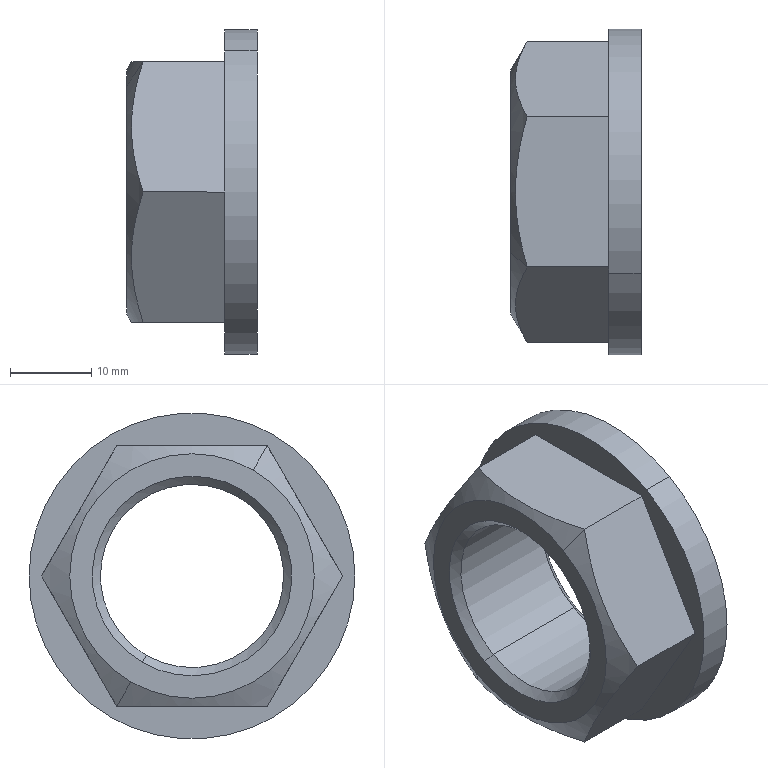Part | SolidWorks | features BaseBody 1 | 1 solid | 19 faces | box 16 x 40 x 40 mm | volume 9123 mm3 | plane 9 | cone 6 | cylinder 4 | commonest cylinder face diameters 22.5 x2 40 x2
STEP:
#1=CARTESIAN_POINT('',(-53.,10.,-17.321));
#2=VERTEX_POINT('',#1);
#3=CARTESIAN_POINT('',(-53.,-10.,17.321));
#4=VERTEX_POINT('',#3);
#5=CARTESIAN_POINT('',(-53.,0.,0.));
#6=DIRECTION('',(1.,0.,0.));
#7=DIRECTION('',(0.,0.5,-0.866));
#8=AXIS2_PLACEMENT_3D('',#5,#6,#7);
#9=CIRCLE('',#8,20.);
#10=EDGE_CURVE('',#2,#4,#9,.T.);
#11=ORIENTED_EDGE('',*,*,#10,.T.);
#12=CARTESIAN_POINT('',(-49.,-10.,17.321));
#13=VERTEX_POINT('',#12);
#14=CARTESIAN_POINT('',(-53.,-10.,17.321));
#15=DIRECTION('',(1.,0.,0.));
#16=VECTOR('',#15,1000.);
#17=LINE('',#14,#16);
#18=EDGE_CURVE('',#4,#13,#17,.T.);
#19=ORIENTED_EDGE('',*,*,#18,.T.);
#20=CARTESIAN_POINT('',(-49.,10.,-17.321));
#21=VERTEX_POINT('',#20);
#22=CARTESIAN_POINT('',(-49.,0.,0.));
#23=DIRECTION('',(1.,0.,0.));
#24=DIRECTION('',(0.,0.5,-0.866));
#25=AXIS2_PLACEMENT_3D('',#22,#23,#24);
#26=CIRCLE('',#25,20.);
#27=EDGE_CURVE('',#21,#13,#26,.T.);
#28=ORIENTED_EDGE('',*,*,#27,.F.);
#29=CARTESIAN_POINT('',(-53.,10.,-17.321));
#30=DIRECTION('',(1.,0.,0.));
#31=VECTOR('',#30,1000.);
#32=LINE('',#29,#31);
#33=EDGE_CURVE('',#2,#21,#32,.T.);
#34=ORIENTED_EDGE('',*,*,#33,.F.);
#35=EDGE_LOOP('',(#11,#19,#28,#34));
#36=FACE_OUTER_BOUND('',#35,.T.);
#37=CARTESIAN_POINT('',(-53.,0.,0.));
#38=DIRECTION('',(1.,0.,0.));
#39=DIRECTION('',(0.,0.5,-0.866));
#40=AXIS2_PLACEMENT_3D('',#37,#38,#39);
#41=CYLINDRICAL_SURFACE('',#40,20.);
#42=ADVANCED_FACE('',(#36),#41,.T.);
#43=CARTESIAN_POINT('',(-64.,5.625,-9.743));
#44=VERTEX_POINT('',#43);
#45=CARTESIAN_POINT('',(-64.,-5.625,9.743));
#46=VERTEX_POINT('',#45);
#47=CARTESIAN_POINT('',(-64.,0.,0.));
#48=DIRECTION('',(-1.,0.,0.));
#49=DIRECTION('',(0.,0.5,-0.866));
#50=AXIS2_PLACEMENT_3D('',#47,#48,#49);
#51=CIRCLE('',#50,11.25);
#52=EDGE_CURVE('',#44,#46,#51,.T.);
#53=ORIENTED_EDGE('',*,*,#52,.F.);
#54=CARTESIAN_POINT('',(-65.,6.125,-10.609));
#55=VERTEX_POINT('',#54);
#56=CARTESIAN_POINT('',(-65.,6.125,-10.609));
#57=DIRECTION('',(-0.7071,0.3536,-0.6124));
#58=VECTOR('',#57,1000.);
#59=LINE('',#56,#58);
#60=EDGE_CURVE('',#44,#55,#59,.T.);
#61=ORIENTED_EDGE('',*,*,#60,.T.);
#62=CARTESIAN_POINT('',(-65.,-6.125,10.609));
#63=VERTEX_POINT('',#62);
#64=CARTESIAN_POINT('',(-65.,0.,0.));
#65=DIRECTION('',(1.,0.,0.));
#66=DIRECTION('',(0.,0.5,-0.866));
#67=AXIS2_PLACEMENT_3D('',#64,#65,#66);
#68=CIRCLE('',#67,12.25);
#69=EDGE_CURVE('',#63,#55,#68,.T.);
#70=ORIENTED_EDGE('',*,*,#69,.F.);
#71=CARTESIAN_POINT('',(-65.,-6.125,10.609));
#72=DIRECTION('',(-0.7071,-0.3536,0.6124));
#73=VECTOR('',#72,1000.);
#74=LINE('',#71,#73);
#75=EDGE_CURVE('',#46,#63,#74,.T.);
#76=ORIENTED_EDGE('',*,*,#75,.F.);
#77=EDGE_LOOP('',(#53,#61,#70,#76));
#78=FACE_OUTER_BOUND('',#77,.T.);
#79=CARTESIAN_POINT('',(-65.,0.,0.));
#80=DIRECTION('',(-1.,0.,0.));
#81=DIRECTION('',(0.,-0.5,0.866));
#82=AXIS2_PLACEMENT_3D('',#79,#80,#81);
#83=CONICAL_SURFACE('',#82,12.25,0.7854);
#84=ADVANCED_FACE('',(#78),#83,.F.);
#85=CARTESIAN_POINT('',(-50.,-5.625,9.743));
#86=VERTEX_POINT('',#85);
#87=CARTESIAN_POINT('',(-50.,5.625,-9.743));
#88=VERTEX_POINT('',#87);
#89=CARTESIAN_POINT('',(-50.,0.,0.));
#90=DIRECTION('',(1.,0.,0.));
#91=DIRECTION('',(0.,0.5,-0.866));
#92=AXIS2_PLACEMENT_3D('',#89,#90,#91);
#93=CIRCLE('',#92,11.25);
#94=EDGE_CURVE('',#86,#88,#93,.T.);
#95=ORIENTED_EDGE('',*,*,#94,.F.);
#96=CARTESIAN_POINT('',(-49.,-6.125,10.609));
#97=VERTEX_POINT('',#96);
#98=CARTESIAN_POINT('',(-50.,-5.625,9.743));
#99=DIRECTION('',(0.7071,-0.3536,0.6124));
#100=VECTOR('',#99,1000.);
#101=LINE('',#98,#100);
#102=EDGE_CURVE('',#86,#97,#101,.T.);
#103=ORIENTED_EDGE('',*,*,#102,.T.);
#104=CARTESIAN_POINT('',(-49.,6.125,-10.609));
#105=VERTEX_POINT('',#104);
#106=CARTESIAN_POINT('',(-49.,0.,0.));
#107=DIRECTION('',(-1.,0.,0.));
#108=DIRECTION('',(0.,0.5,-0.866));
#109=AXIS2_PLACEMENT_3D('',#106,#107,#108);
#110=CIRCLE('',#109,12.25);
#111=EDGE_CURVE('',#105,#97,#110,.T.);
#112=ORIENTED_EDGE('',*,*,#111,.F.);
#113=CARTESIAN_POINT('',(-50.,5.625,-9.743));
#114=DIRECTION('',(0.7071,0.3536,-0.6124));
#115=VECTOR('',#114,1000.);
#116=LINE('',#113,#115);
#117=EDGE_CURVE('',#88,#105,#116,.T.);
#118=ORIENTED_EDGE('',*,*,#117,.F.);
#119=EDGE_LOOP('',(#95,#103,#112,#118));
#120=FACE_OUTER_BOUND('',#119,.T.);
#121=CARTESIAN_POINT('',(-50.,0.,0.));
#122=DIRECTION('',(1.,0.,0.));
#123=DIRECTION('',(0.,0.5,-0.866));
#124=AXIS2_PLACEMENT_3D('',#121,#122,#123);
#125=CONICAL_SURFACE('',#124,11.25,0.7854);
#126=ADVANCED_FACE('',(#120),#125,.F.);
#127=CARTESIAN_POINT('',(-65.,-7.506,13.));
#128=VERTEX_POINT('',#127);
#129=CARTESIAN_POINT('',(-65.,7.506,-13.));
#130=VERTEX_POINT('',#129);
#131=CARTESIAN_POINT('',(-65.,0.,0.));
#132=DIRECTION('',(-1.,0.,0.));
#133=DIRECTION('',(0.,-0.5,0.866));
#134=AXIS2_PLACEMENT_3D('',#131,#132,#133);
#135=CIRCLE('',#134,15.011);
#136=EDGE_CURVE('',#128,#130,#135,.T.);
#137=ORIENTED_EDGE('',*,*,#136,.F.);
#138=CARTESIAN_POINT('',(-63.,-9.238,16.));
#139=VERTEX_POINT('',#138);
#140=CARTESIAN_POINT('',(-65.,-7.506,13.));
#141=DIRECTION('',(0.5,-0.433,0.75));
#142=VECTOR('',#141,1000.);
#143=LINE('',#140,#142);
#144=EDGE_CURVE('',#128,#139,#143,.T.);
#145=ORIENTED_EDGE('',*,*,#144,.T.);
#146=CARTESIAN_POINT('',(-63.,9.238,16.));
#147=VERTEX_POINT('',#146);
#148=CARTESIAN_POINT('',(-63.,-9.238,16.));
#149=CARTESIAN_POINT('',(-63.435,-7.729,16.));
#150=CARTESIAN_POINT('',(-63.794,-6.21,16.));
#151=CARTESIAN_POINT('',(-64.291,-3.14,16.));
#152=CARTESIAN_POINT('',(-64.428,-1.588,16.));
#153=CARTESIAN_POINT('',(-64.43,0.7677,16.));
#154=CARTESIAN_POINT('',(-64.396,1.557,16.));
#155=CARTESIAN_POINT('',(-64.266,3.118,16.));
#156=CARTESIAN_POINT('',(-64.169,3.893,16.));
#157=CARTESIAN_POINT('',(-63.796,6.205,16.));
#158=CARTESIAN_POINT('',(-63.436,7.727,16.));
#159=CARTESIAN_POINT('',(-63.,9.238,16.));
#160=B_SPLINE_CURVE_WITH_KNOTS('',3,(#148,#149,#150,#151,#152,#153,#154,#155,#156,#157,#158,#159),.UNSPECIFIED.,.F.,.F.,(4,2,2,2,2,4),(0.000000238,0.004665,0.00933,0.01166,0.01399,0.01866),.UNSPECIFIED.);
#161=EDGE_CURVE('',#139,#147,#160,.T.);
#162=ORIENTED_EDGE('',*,*,#161,.T.);
#163=CARTESIAN_POINT('',(-63.,18.475,0.));
#164=VERTEX_POINT('',#163);
#165=CARTESIAN_POINT('',(-63.,9.238,16.));
#166=CARTESIAN_POINT('',(-63.217,9.613,15.349));
#167=CARTESIAN_POINT('',(-63.416,9.992,14.693));
#168=CARTESIAN_POINT('',(-63.769,10.759,13.364));
#169=CARTESIAN_POINT('',(-63.922,11.144,12.698));
#170=CARTESIAN_POINT('',(-64.295,12.301,10.693));
#171=CARTESIAN_POINT('',(-64.429,13.077,9.35));
#172=CARTESIAN_POINT('',(-64.429,14.248,7.322));
#173=CARTESIAN_POINT('',(-64.396,14.64,6.644));
#174=CARTESIAN_POINT('',(-64.264,15.425,5.283));
#175=CARTESIAN_POINT('',(-64.166,15.815,4.607));
#176=CARTESIAN_POINT('',(-63.79,16.972,2.603));
#177=CARTESIAN_POINT('',(-63.431,17.729,1.293));
#178=CARTESIAN_POINT('',(-63.,18.475,0.));
#179=B_SPLINE_CURVE_WITH_KNOTS('',3,(#165,#166,#167,#168,#169,#170,#171,#172,#173,#174,#175,#176,#177,#178),.UNSPECIFIED.,.F.,.F.,(4,2,2,2,2,2,4),(0.01639,0.01873,0.02107,0.02574,0.02808,0.03041,0.03509),.UNSPECIFIED.);
#180=EDGE_CURVE('',#147,#164,#179,.T.);
#181=ORIENTED_EDGE('',*,*,#180,.T.);
#182=CARTESIAN_POINT('',(-63.,9.238,-16.));
#183=VERTEX_POINT('',#182);
#184=CARTESIAN_POINT('',(-63.,18.475,0.));
#185=CARTESIAN_POINT('',(-63.435,17.721,-1.306));
#186=CARTESIAN_POINT('',(-63.794,16.961,-2.622));
#187=CARTESIAN_POINT('',(-64.291,15.426,-5.281));
#188=CARTESIAN_POINT('',(-64.428,14.651,-6.624));
#189=CARTESIAN_POINT('',(-64.43,13.473,-8.665));
#190=CARTESIAN_POINT('',(-64.396,13.078,-9.348));
#191=CARTESIAN_POINT('',(-64.266,12.298,-10.7));
#192=CARTESIAN_POINT('',(-64.169,11.91,-11.371));
#193=CARTESIAN_POINT('',(-63.796,10.754,-13.373));
#194=CARTESIAN_POINT('',(-63.436,9.993,-14.692));
#195=CARTESIAN_POINT('',(-63.,9.238,-16.));
#196=B_SPLINE_CURVE_WITH_KNOTS('',3,(#184,#185,#186,#187,#188,#189,#190,#191,#192,#193,#194,#195),.UNSPECIFIED.,.F.,.F.,(4,2,2,2,2,4),(0.000000238,0.004665,0.00933,0.01166,0.01399,0.01866),.UNSPECIFIED.);
#197=EDGE_CURVE('',#164,#183,#196,.T.);
#198=ORIENTED_EDGE('',*,*,#197,.T.);
#199=CARTESIAN_POINT('',(-65.,7.506,-13.));
#200=DIRECTION('',(0.5,0.433,-0.75));
#201=VECTOR('',#200,1000.);
#202=LINE('',#199,#201);
#203=EDGE_CURVE('',#130,#183,#202,.T.);
#204=ORIENTED_EDGE('',*,*,#203,.F.);
#205=EDGE_LOOP('',(#137,#145,#162,#181,#198,#204));
#206=FACE_OUTER_BOUND('',#205,.T.);
#207=CARTESIAN_POINT('',(-65.,0.,0.));
#208=DIRECTION('',(1.,0.,0.));
#209=DIRECTION('',(0.,0.5,-0.866));
#210=AXIS2_PLACEMENT_3D('',#207,#208,#209);
#211=CONICAL_SURFACE('',#210,15.011,1.047);
#212=ADVANCED_FACE('',(#206),#211,.T.);
#213=ORIENTED_EDGE('',*,*,#94,.T.);
#214=CARTESIAN_POINT('',(-49.,5.625,-9.743));
#215=DIRECTION('',(-1.,0.,0.));
#216=VECTOR('',#215,1000.);
#217=LINE('',#214,#216);
#218=EDGE_CURVE('',#88,#44,#217,.T.);
#219=ORIENTED_EDGE('',*,*,#218,.T.);
#220=ORIENTED_EDGE('',*,*,#52,.T.);
#221=CARTESIAN_POINT('',(-49.,-5.625,9.743));
#222=DIRECTION('',(-1.,0.,0.));
#223=VECTOR('',#222,1000.);
#224=LINE('',#221,#223);
#225=EDGE_CURVE('',#86,#46,#224,.T.);
#226=ORIENTED_EDGE('',*,*,#225,.F.);
#227=EDGE_LOOP('',(#213,#219,#220,#226));
#228=FACE_OUTER_BOUND('',#227,.T.);
#229=CARTESIAN_POINT('',(-49.,0.,0.));
#230=DIRECTION('',(-1.,0.,0.));
#231=DIRECTION('',(0.,-0.5,0.866));
#232=AXIS2_PLACEMENT_3D('',#229,#230,#231);
#233=CYLINDRICAL_SURFACE('',#232,11.25);
#234=ADVANCED_FACE('',(#228),#233,.F.);
#235=CARTESIAN_POINT('',(-53.,-9.238,-16.));
#236=VERTEX_POINT('',#235);
#237=CARTESIAN_POINT('',(-53.,9.238,-16.));
#238=VERTEX_POINT('',#237);
#239=CARTESIAN_POINT('',(-53.,-9.238,-16.));
#240=DIRECTION('',(0.,1.,0.));
#241=VECTOR('',#240,1000.);
#242=LINE('',#239,#241);
#243=EDGE_CURVE('',#236,#238,#242,.T.);
#244=ORIENTED_EDGE('',*,*,#243,.F.);
#245=CARTESIAN_POINT('',(-63.,-9.238,-16.));
#246=VERTEX_POINT('',#245);
#247=CARTESIAN_POINT('',(-49.,-9.238,-16.));
#248=DIRECTION('',(-1.,0.,0.));
#249=VECTOR('',#248,1000.);
#250=LINE('',#247,#249);
#251=EDGE_CURVE('',#236,#246,#250,.T.);
#252=ORIENTED_EDGE('',*,*,#251,.T.);
#253=CARTESIAN_POINT('',(-63.,9.238,-16.));
#254=CARTESIAN_POINT('',(-63.435,7.729,-16.));
#255=CARTESIAN_POINT('',(-63.794,6.21,-16.));
#256=CARTESIAN_POINT('',(-64.291,3.14,-16.));
#257=CARTESIAN_POINT('',(-64.428,1.588,-16.));
#258=CARTESIAN_POINT('',(-64.43,-0.7677,-16.));
#259=CARTESIAN_POINT('',(-64.396,-1.557,-16.));
#260=CARTESIAN_POINT('',(-64.266,-3.118,-16.));
#261=CARTESIAN_POINT('',(-64.169,-3.893,-16.));
#262=CARTESIAN_POINT('',(-63.796,-6.205,-16.));
#263=CARTESIAN_POINT('',(-63.436,-7.727,-16.));
#264=CARTESIAN_POINT('',(-63.,-9.238,-16.));
#265=B_SPLINE_CURVE_WITH_KNOTS('',3,(#253,#254,#255,#256,#257,#258,#259,#260,#261,#262,#263,#264),.UNSPECIFIED.,.F.,.F.,(4,2,2,2,2,4),(0.000000238,0.004665,0.00933,0.01166,0.01399,0.01866),.UNSPECIFIED.);
#266=EDGE_CURVE('',#183,#246,#265,.T.);
#267=ORIENTED_EDGE('',*,*,#266,.F.);
#268=CARTESIAN_POINT('',(-49.,9.238,-16.));
#269=DIRECTION('',(-1.,0.,0.));
#270=VECTOR('',#269,1000.);
#271=LINE('',#268,#270);
#272=EDGE_CURVE('',#238,#183,#271,.T.);
#273=ORIENTED_EDGE('',*,*,#272,.F.);
#274=EDGE_LOOP('',(#244,#252,#267,#273));
#275=FACE_OUTER_BOUND('',#274,.T.);
#276=CARTESIAN_POINT('',(-49.,-9.238,-16.));
#277=DIRECTION('',(0.,0.,1.));
#278=DIRECTION('',(0.,-1.,0.));
#279=AXIS2_PLACEMENT_3D('',#276,#277,#278);
#280=PLANE('',#279);
#281=ADVANCED_FACE('',(#275),#280,.F.);
#282=CARTESIAN_POINT('',(-53.,18.475,0.));
#283=VERTEX_POINT('',#282);
#284=CARTESIAN_POINT('',(-53.,9.238,-16.));
#285=DIRECTION('',(0.,0.5,0.866));
#286=VECTOR('',#285,1000.);
#287=LINE('',#284,#286);
#288=EDGE_CURVE('',#238,#283,#287,.T.);
#289=ORIENTED_EDGE('',*,*,#288,.F.);
#290=ORIENTED_EDGE('',*,*,#272,.T.);
#291=ORIENTED_EDGE('',*,*,#197,.F.);
#292=CARTESIAN_POINT('',(-49.,18.475,0.));
#293=DIRECTION('',(-1.,0.,0.));
#294=VECTOR('',#293,1000.);
#295=LINE('',#292,#294);
#296=EDGE_CURVE('',#283,#164,#295,.T.);
#297=ORIENTED_EDGE('',*,*,#296,.F.);
#298=EDGE_LOOP('',(#289,#290,#291,#297));
#299=FACE_OUTER_BOUND('',#298,.T.);
#300=CARTESIAN_POINT('',(-49.,9.238,-16.));
#301=DIRECTION('',(0.,-0.866,0.5));
#302=DIRECTION('',(0.,-0.5,-0.866));
#303=AXIS2_PLACEMENT_3D('',#300,#301,#302);
#304=PLANE('',#303);
#305=ADVANCED_FACE('',(#299),#304,.F.);
#306=CARTESIAN_POINT('',(-53.,9.238,16.));
#307=VERTEX_POINT('',#306);
#308=CARTESIAN_POINT('',(-53.,18.475,0.));
#309=DIRECTION('',(0.,-0.5,0.866));
#310=VECTOR('',#309,1000.);
#311=LINE('',#308,#310);
#312=EDGE_CURVE('',#283,#307,#311,.T.);
#313=ORIENTED_EDGE('',*,*,#312,.F.);
#314=ORIENTED_EDGE('',*,*,#296,.T.);
#315=ORIENTED_EDGE('',*,*,#180,.F.);
#316=CARTESIAN_POINT('',(-49.,9.238,16.));
#317=DIRECTION('',(-1.,0.,0.));
#318=VECTOR('',#317,1000.);
#319=LINE('',#316,#318);
#320=EDGE_CURVE('',#307,#147,#319,.T.);
#321=ORIENTED_EDGE('',*,*,#320,.F.);
#322=EDGE_LOOP('',(#313,#314,#315,#321));
#323=FACE_OUTER_BOUND('',#322,.T.);
#324=CARTESIAN_POINT('',(-49.,18.475,0.));
#325=DIRECTION('',(0.,-0.866,-0.5));
#326=DIRECTION('',(-1.,0.,0.));
#327=AXIS2_PLACEMENT_3D('',#324,#325,#326);
#328=PLANE('',#327);
#329=ADVANCED_FACE('',(#323),#328,.F.);
#330=CARTESIAN_POINT('',(-53.,-9.238,16.));
#331=VERTEX_POINT('',#330);
#332=CARTESIAN_POINT('',(-53.,9.238,16.));
#333=DIRECTION('',(0.,-1.,0.));
#334=VECTOR('',#333,1000.);
#335=LINE('',#332,#334);
#336=EDGE_CURVE('',#307,#331,#335,.T.);
#337=ORIENTED_EDGE('',*,*,#336,.F.);
#338=ORIENTED_EDGE('',*,*,#320,.T.);
#339=ORIENTED_EDGE('',*,*,#161,.F.);
#340=CARTESIAN_POINT('',(-49.,-9.238,16.));
#341=DIRECTION('',(-1.,0.,0.));
#342=VECTOR('',#341,1000.);
#343=LINE('',#340,#342);
#344=EDGE_CURVE('',#331,#139,#343,.T.);
#345=ORIENTED_EDGE('',*,*,#344,.F.);
#346=EDGE_LOOP('',(#337,#338,#339,#345));
#347=FACE_OUTER_BOUND('',#346,.T.);
#348=CARTESIAN_POINT('',(-49.,9.238,16.));
#349=DIRECTION('',(0.,0.,-1.));
#350=DIRECTION('',(0.,1.,0.));
#351=AXIS2_PLACEMENT_3D('',#348,#349,#350);
#352=PLANE('',#351);
#353=ADVANCED_FACE('',(#347),#352,.F.);
#354=CARTESIAN_POINT('',(-53.,-18.475,0.));
#355=VERTEX_POINT('',#354);
#356=CARTESIAN_POINT('',(-53.,-9.238,16.));
#357=DIRECTION('',(0.,-0.5,-0.866));
#358=VECTOR('',#357,1000.);
#359=LINE('',#356,#358);
#360=EDGE_CURVE('',#331,#355,#359,.T.);
#361=ORIENTED_EDGE('',*,*,#360,.F.);
#362=ORIENTED_EDGE('',*,*,#344,.T.);
#363=CARTESIAN_POINT('',(-63.,-18.475,0.));
#364=VERTEX_POINT('',#363);
#365=CARTESIAN_POINT('',(-63.,-18.475,0.));
#366=CARTESIAN_POINT('',(-63.435,-17.721,1.306));
#367=CARTESIAN_POINT('',(-63.794,-16.961,2.622));
#368=CARTESIAN_POINT('',(-64.291,-15.426,5.281));
#369=CARTESIAN_POINT('',(-64.428,-14.651,6.624));
#370=CARTESIAN_POINT('',(-64.43,-13.473,8.665));
#371=CARTESIAN_POINT('',(-64.396,-13.078,9.348));
#372=CARTESIAN_POINT('',(-64.266,-12.298,10.7));
#373=CARTESIAN_POINT('',(-64.169,-11.91,11.371));
#374=CARTESIAN_POINT('',(-63.796,-10.754,13.373));
#375=CARTESIAN_POINT('',(-63.436,-9.993,14.692));
#376=CARTESIAN_POINT('',(-63.,-9.238,16.));
#377=B_SPLINE_CURVE_WITH_KNOTS('',3,(#365,#366,#367,#368,#369,#370,#371,#372,#373,#374,#375,#376),.UNSPECIFIED.,.F.,.F.,(4,2,2,2,2,4),(0.000000238,0.004665,0.00933,0.01166,0.01399,0.01866),.UNSPECIFIED.);
#378=EDGE_CURVE('',#364,#139,#377,.T.);
#379=ORIENTED_EDGE('',*,*,#378,.F.);
#380=CARTESIAN_POINT('',(-49.,-18.475,0.));
#381=DIRECTION('',(-1.,0.,0.));
#382=VECTOR('',#381,1000.);
#383=LINE('',#380,#382);
#384=EDGE_CURVE('',#355,#364,#383,.T.);
#385=ORIENTED_EDGE('',*,*,#384,.F.);
#386=EDGE_LOOP('',(#361,#362,#379,#385));
#387=FACE_OUTER_BOUND('',#386,.T.);
#388=CARTESIAN_POINT('',(-49.,-9.238,16.));
#389=DIRECTION('',(0.,0.866,-0.5));
#390=DIRECTION('',(0.,0.5,0.866));
#391=AXIS2_PLACEMENT_3D('',#388,#389,#390);
#392=PLANE('',#391);
#393=ADVANCED_FACE('',(#387),#392,.F.);
#394=CARTESIAN_POINT('',(-53.,-18.475,0.));
#395=DIRECTION('',(0.,0.5,-0.866));
#396=VECTOR('',#395,1000.);
#397=LINE('',#394,#396);
#398=EDGE_CURVE('',#355,#236,#397,.T.);
#399=ORIENTED_EDGE('',*,*,#398,.F.);
#400=ORIENTED_EDGE('',*,*,#384,.T.);
#401=CARTESIAN_POINT('',(-63.,-9.238,-16.));
#402=CARTESIAN_POINT('',(-63.431,-9.984,-14.707));
#403=CARTESIAN_POINT('',(-63.79,-10.741,-13.397));
#404=CARTESIAN_POINT('',(-64.166,-11.898,-11.393));
#405=CARTESIAN_POINT('',(-64.264,-12.288,-10.717));
#406=CARTESIAN_POINT('',(-64.396,-13.073,-9.356));
#407=CARTESIAN_POINT('',(-64.429,-13.465,-8.678));
#408=CARTESIAN_POINT('',(-64.429,-14.636,-6.65));
#409=CARTESIAN_POINT('',(-64.295,-15.411,-5.307));
#410=CARTESIAN_POINT('',(-63.922,-16.569,-3.302));
#411=CARTESIAN_POINT('',(-63.769,-16.954,-2.636));
#412=CARTESIAN_POINT('',(-63.416,-17.72,-1.307));
#413=CARTESIAN_POINT('',(-63.217,-18.1,-0.6506));
#414=CARTESIAN_POINT('',(-63.,-18.475,0.));
#415=B_SPLINE_CURVE_WITH_KNOTS('',3,(#401,#402,#403,#404,#405,#406,#407,#408,#409,#410,#411,#412,#413,#414),.UNSPECIFIED.,.F.,.F.,(4,2,2,2,2,2,4),(0.006866,0.01153,0.01386,0.01619,0.02085,0.02318,0.02551),.UNSPECIFIED.);
#416=EDGE_CURVE('',#246,#364,#415,.T.);
#417=ORIENTED_EDGE('',*,*,#416,.F.);
#418=ORIENTED_EDGE('',*,*,#251,.F.);
#419=EDGE_LOOP('',(#399,#400,#417,#418));
#420=FACE_OUTER_BOUND('',#419,.T.);
#421=CARTESIAN_POINT('',(-49.,-18.475,0.));
#422=DIRECTION('',(0.,0.866,0.5));
#423=DIRECTION('',(0.,-0.5,0.866));
#424=AXIS2_PLACEMENT_3D('',#421,#422,#423);
#425=PLANE('',#424);
#426=ADVANCED_FACE('',(#420),#425,.F.);
#427=ORIENTED_EDGE('',*,*,#69,.T.);
#428=CARTESIAN_POINT('',(-65.,0.,0.));
#429=DIRECTION('',(1.,0.,0.));
#430=DIRECTION('',(0.,0.5,-0.866));
#431=AXIS2_PLACEMENT_3D('',#428,#429,#430);
#432=CIRCLE('',#431,12.25);
#433=EDGE_CURVE('',#55,#63,#432,.T.);
#434=ORIENTED_EDGE('',*,*,#433,.T.);
#435=EDGE_LOOP('',(#427,#434));
#436=FACE_BOUND('',#435,.T.);
#437=CARTESIAN_POINT('',(-65.,0.,0.));
#438=DIRECTION('',(-1.,0.,0.));
#439=DIRECTION('',(0.,-0.5,0.866));
#440=AXIS2_PLACEMENT_3D('',#437,#438,#439);
#441=CIRCLE('',#440,15.011);
#442=EDGE_CURVE('',#130,#128,#441,.T.);
#443=ORIENTED_EDGE('',*,*,#442,.T.);
#444=ORIENTED_EDGE('',*,*,#136,.T.);
#445=EDGE_LOOP('',(#443,#444));
#446=FACE_OUTER_BOUND('',#445,.T.);
#447=CARTESIAN_POINT('',(-65.,9.238,-16.));
#448=DIRECTION('',(1.,0.,0.));
#449=DIRECTION('',(0.,0.5,-0.866));
#450=AXIS2_PLACEMENT_3D('',#447,#448,#449);
#451=PLANE('',#450);
#452=ADVANCED_FACE('',(#436,#446),#451,.F.);
#453=ORIENTED_EDGE('',*,*,#111,.T.);
#454=CARTESIAN_POINT('',(-49.,0.,0.));
#455=DIRECTION('',(-1.,0.,0.));
#456=DIRECTION('',(0.,0.5,-0.866));
#457=AXIS2_PLACEMENT_3D('',#454,#455,#456);
#458=CIRCLE('',#457,12.25);
#459=EDGE_CURVE('',#97,#105,#458,.T.);
#460=ORIENTED_EDGE('',*,*,#459,.T.);
#461=EDGE_LOOP('',(#453,#460));
#462=FACE_BOUND('',#461,.T.);
#463=ORIENTED_EDGE('',*,*,#27,.T.);
#464=CARTESIAN_POINT('',(-49.,0.,0.));
#465=DIRECTION('',(1.,0.,0.));
#466=DIRECTION('',(0.,0.5,-0.866));
#467=AXIS2_PLACEMENT_3D('',#464,#465,#466);
#468=CIRCLE('',#467,20.);
#469=EDGE_CURVE('',#13,#21,#468,.T.);
#470=ORIENTED_EDGE('',*,*,#469,.T.);
#471=EDGE_LOOP('',(#463,#470));
#472=FACE_OUTER_BOUND('',#471,.T.);
#473=CARTESIAN_POINT('',(-49.,9.238,-16.));
#474=DIRECTION('',(1.,0.,0.));
#475=DIRECTION('',(0.,0.5,-0.866));
#476=AXIS2_PLACEMENT_3D('',#473,#474,#475);
#477=PLANE('',#476);
#478=ADVANCED_FACE('',(#462,#472),#477,.T.);
#479=ORIENTED_EDGE('',*,*,#218,.F.);
#480=CARTESIAN_POINT('',(-50.,0.,0.));
#481=DIRECTION('',(1.,0.,0.));
#482=DIRECTION('',(0.,0.5,-0.866));
#483=AXIS2_PLACEMENT_3D('',#480,#481,#482);
#484=CIRCLE('',#483,11.25);
#485=EDGE_CURVE('',#88,#86,#484,.T.);
#486=ORIENTED_EDGE('',*,*,#485,.T.);
#487=ORIENTED_EDGE('',*,*,#225,.T.);
#488=CARTESIAN_POINT('',(-64.,0.,0.));
#489=DIRECTION('',(-1.,0.,0.));
#490=DIRECTION('',(0.,0.5,-0.866));
#491=AXIS2_PLACEMENT_3D('',#488,#489,#490);
#492=CIRCLE('',#491,11.25);
#493=EDGE_CURVE('',#46,#44,#492,.T.);
#494=ORIENTED_EDGE('',*,*,#493,.T.);
#495=EDGE_LOOP('',(#479,#486,#487,#494));
#496=FACE_OUTER_BOUND('',#495,.T.);
#497=CARTESIAN_POINT('',(-49.,0.,0.));
#498=DIRECTION('',(-1.,0.,0.));
#499=DIRECTION('',(0.,-0.5,0.866));
#500=AXIS2_PLACEMENT_3D('',#497,#498,#499);
#501=CYLINDRICAL_SURFACE('',#500,11.25);
#502=ADVANCED_FACE('',(#496),#501,.F.);
#503=ORIENTED_EDGE('',*,*,#144,.F.);
#504=ORIENTED_EDGE('',*,*,#442,.F.);
#505=ORIENTED_EDGE('',*,*,#203,.T.);
#506=ORIENTED_EDGE('',*,*,#266,.T.);
#507=ORIENTED_EDGE('',*,*,#416,.T.);
#508=ORIENTED_EDGE('',*,*,#378,.T.);
#509=EDGE_LOOP('',(#503,#504,#505,#506,#507,#508));
#510=FACE_OUTER_BOUND('',#509,.T.);
#511=CARTESIAN_POINT('',(-65.,0.,0.));
#512=DIRECTION('',(1.,0.,0.));
#513=DIRECTION('',(0.,0.5,-0.866));
#514=AXIS2_PLACEMENT_3D('',#511,#512,#513);
#515=CONICAL_SURFACE('',#514,15.011,1.047);
#516=ADVANCED_FACE('',(#510),#515,.T.);
#517=ORIENTED_EDGE('',*,*,#102,.F.);
#518=ORIENTED_EDGE('',*,*,#485,.F.);
#519=ORIENTED_EDGE('',*,*,#117,.T.);
#520=ORIENTED_EDGE('',*,*,#459,.F.);
#521=EDGE_LOOP('',(#517,#518,#519,#520));
#522=FACE_OUTER_BOUND('',#521,.T.);
#523=CARTESIAN_POINT('',(-50.,0.,0.));
#524=DIRECTION('',(1.,0.,0.));
#525=DIRECTION('',(0.,0.5,-0.866));
#526=AXIS2_PLACEMENT_3D('',#523,#524,#525);
#527=CONICAL_SURFACE('',#526,11.25,0.7854);
#528=ADVANCED_FACE('',(#522),#527,.F.);
#529=ORIENTED_EDGE('',*,*,#60,.F.);
#530=ORIENTED_EDGE('',*,*,#493,.F.);
#531=ORIENTED_EDGE('',*,*,#75,.T.);
#532=ORIENTED_EDGE('',*,*,#433,.F.);
#533=EDGE_LOOP('',(#529,#530,#531,#532));
#534=FACE_OUTER_BOUND('',#533,.T.);
#535=CARTESIAN_POINT('',(-65.,0.,0.));
#536=DIRECTION('',(-1.,0.,0.));
#537=DIRECTION('',(0.,-0.5,0.866));
#538=AXIS2_PLACEMENT_3D('',#535,#536,#537);
#539=CONICAL_SURFACE('',#538,12.25,0.7854);
#540=ADVANCED_FACE('',(#534),#539,.F.);
#541=ORIENTED_EDGE('',*,*,#18,.F.);
#542=CARTESIAN_POINT('',(-53.,0.,0.));
#543=DIRECTION('',(1.,0.,0.));
#544=DIRECTION('',(0.,0.5,-0.866));
#545=AXIS2_PLACEMENT_3D('',#542,#543,#544);
#546=CIRCLE('',#545,20.);
#547=EDGE_CURVE('',#4,#2,#546,.T.);
#548=ORIENTED_EDGE('',*,*,#547,.T.);
#549=ORIENTED_EDGE('',*,*,#33,.T.);
#550=ORIENTED_EDGE('',*,*,#469,.F.);
#551=EDGE_LOOP('',(#541,#548,#549,#550));
#552=FACE_OUTER_BOUND('',#551,.T.);
#553=CARTESIAN_POINT('',(-53.,0.,0.));
#554=DIRECTION('',(1.,0.,0.));
#555=DIRECTION('',(0.,0.5,-0.866));
#556=AXIS2_PLACEMENT_3D('',#553,#554,#555);
#557=CYLINDRICAL_SURFACE('',#556,20.);
#558=ADVANCED_FACE('',(#552),#557,.T.);
#559=ORIENTED_EDGE('',*,*,#398,.T.);
#560=ORIENTED_EDGE('',*,*,#243,.T.);
#561=ORIENTED_EDGE('',*,*,#288,.T.);
#562=ORIENTED_EDGE('',*,*,#312,.T.);
#563=ORIENTED_EDGE('',*,*,#336,.T.);
#564=ORIENTED_EDGE('',*,*,#360,.T.);
#565=EDGE_LOOP('',(#559,#560,#561,#562,#563,#564));
#566=FACE_BOUND('',#565,.T.);
#567=ORIENTED_EDGE('',*,*,#10,.F.);
#568=ORIENTED_EDGE('',*,*,#547,.F.);
#569=EDGE_LOOP('',(#567,#568));
#570=FACE_OUTER_BOUND('',#569,.T.);
#571=CARTESIAN_POINT('',(-53.,0.,0.));
#572=DIRECTION('',(1.,0.,0.));
#573=DIRECTION('',(0.,0.5,-0.866));
#574=AXIS2_PLACEMENT_3D('',#571,#572,#573);
#575=PLANE('',#574);
#576=ADVANCED_FACE('',(#566,#570),#575,.F.);
#577=CLOSED_SHELL('',(#42,#84,#126,#212,#234,#281,#305,#329,#353,#393,#426,#452,#478,#502,#516,#528,#540,#558,#576));
#578=MANIFOLD_SOLID_BREP('',#577);
#579=CARTESIAN_POINT('',(0.,0.,0.));
#580=DIRECTION('',(0.,0.,1.));
#581=DIRECTION('',(1.,0.,0.));
#582=AXIS2_PLACEMENT_3D('',#579,#580,#581);
#583=(LENGTH_UNIT()NAMED_UNIT(*)SI_UNIT(.MILLI.,.METRE.));
#584=UNCERTAINTY_MEASURE_WITH_UNIT(LENGTH_MEASURE(0.00001),#583,'','');
#585=(NAMED_UNIT(*)PLANE_ANGLE_UNIT()SI_UNIT($,.RADIAN.));
#586=(NAMED_UNIT(*)SI_UNIT($,.STERADIAN.)SOLID_ANGLE_UNIT());
#587=(GEOMETRIC_REPRESENTATION_CONTEXT(3)GLOBAL_UNCERTAINTY_ASSIGNED_CONTEXT((#584))GLOBAL_UNIT_ASSIGNED_CONTEXT((#583,#585,#586))REPRESENTATION_CONTEXT('',''));
#588=ADVANCED_BREP_SHAPE_REPRESENTATION('',(#578,#582),#587);